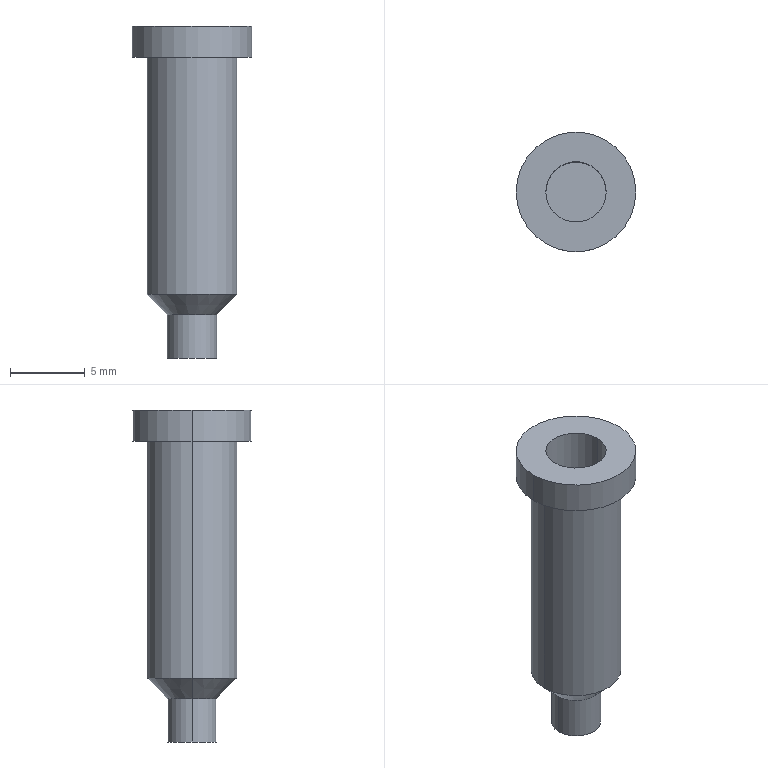Part | NX | features solid 2 | 1 solid | 14 faces | box 8 x 8 x 22.2 mm | volume 371.979 mm3 | cylinder 8 | plane 4 | cone 2 | commonest cylinder face diameters 3.3 x2 4.04 x2 6 x2 8 x2
STEP:
#1=CARTESIAN_POINT('',(-284.273,891.104,-19.1));
#2=VERTEX_POINT('',#1);
#3=CARTESIAN_POINT('',(-287.573,891.104,-19.1));
#4=VERTEX_POINT('',#3);
#5=CARTESIAN_POINT('',(-285.923,891.104,-19.1));
#6=DIRECTION('',(0.,0.,1.));
#7=DIRECTION('',(1.,0.,0.));
#8=AXIS2_PLACEMENT_3D('',#5,#6,#7);
#9=CIRCLE('',#8,1.65);
#10=EDGE_CURVE('',#2,#4,#9,.T.);
#11=ORIENTED_EDGE('',*,*,#10,.F.);
#12=CARTESIAN_POINT('',(-285.923,891.104,-19.1));
#13=DIRECTION('',(0.,0.,1.));
#14=DIRECTION('',(-1.,0.,0.));
#15=AXIS2_PLACEMENT_3D('',#12,#13,#14);
#16=CIRCLE('',#15,1.65);
#17=EDGE_CURVE('',#4,#2,#16,.T.);
#18=ORIENTED_EDGE('',*,*,#17,.F.);
#19=EDGE_LOOP('',(#11,#18));
#20=FACE_BOUND('',#19,.T.);
#21=CARTESIAN_POINT('',(-285.923,891.104,-19.1));
#22=DIRECTION('',(0.,0.,-1.));
#23=DIRECTION('',(-1.,0.,0.));
#24=AXIS2_PLACEMENT_3D('',#21,#22,#23);
#25=PLANE('',#24);
#26=ADVANCED_FACE('',(#20),#25,.T.);
#27=ORIENTED_EDGE('',*,*,#17,.T.);
#28=CARTESIAN_POINT('',(-284.273,891.104,-16.2));
#29=VERTEX_POINT('',#28);
#30=CARTESIAN_POINT('',(-284.273,891.104,-19.1));
#31=DIRECTION('',(0.,0.,1.));
#32=VECTOR('',#31,1000.);
#33=LINE('',#30,#32);
#34=EDGE_CURVE('',#29,#2,#33,.F.);
#35=ORIENTED_EDGE('',*,*,#34,.F.);
#36=CARTESIAN_POINT('',(-287.573,891.104,-16.2));
#37=VERTEX_POINT('',#36);
#38=CARTESIAN_POINT('',(-285.923,891.104,-16.2));
#39=DIRECTION('',(0.,0.,-1.));
#40=DIRECTION('',(1.,0.,0.));
#41=AXIS2_PLACEMENT_3D('',#38,#39,#40);
#42=CIRCLE('',#41,1.65);
#43=EDGE_CURVE('',#29,#37,#42,.T.);
#44=ORIENTED_EDGE('',*,*,#43,.T.);
#45=CARTESIAN_POINT('',(-287.573,891.104,-19.1));
#46=DIRECTION('',(0.,0.,1.));
#47=VECTOR('',#46,1000.);
#48=LINE('',#45,#47);
#49=EDGE_CURVE('',#4,#37,#48,.T.);
#50=ORIENTED_EDGE('',*,*,#49,.F.);
#51=EDGE_LOOP('',(#27,#35,#44,#50));
#52=FACE_BOUND('',#51,.T.);
#53=CARTESIAN_POINT('',(-285.923,891.104,4.21));
#54=DIRECTION('',(0.,0.,-1.));
#55=DIRECTION('',(-1.,0.,0.));
#56=AXIS2_PLACEMENT_3D('',#53,#54,#55);
#57=CYLINDRICAL_SURFACE('',#56,1.65);
#58=ADVANCED_FACE('',(#52),#57,.T.);
#59=CARTESIAN_POINT('',(-285.923,891.104,-16.2));
#60=DIRECTION('',(0.,0.,-1.));
#61=DIRECTION('',(-1.,0.,0.));
#62=AXIS2_PLACEMENT_3D('',#59,#60,#61);
#63=CIRCLE('',#62,1.65);
#64=EDGE_CURVE('',#37,#29,#63,.T.);
#65=ORIENTED_EDGE('',*,*,#64,.T.);
#66=ORIENTED_EDGE('',*,*,#34,.T.);
#67=ORIENTED_EDGE('',*,*,#10,.T.);
#68=ORIENTED_EDGE('',*,*,#49,.T.);
#69=EDGE_LOOP('',(#65,#66,#67,#68));
#70=FACE_BOUND('',#69,.T.);
#71=CARTESIAN_POINT('',(-285.923,891.104,4.21));
#72=DIRECTION('',(0.,0.,-1.));
#73=DIRECTION('',(-1.,0.,0.));
#74=AXIS2_PLACEMENT_3D('',#71,#72,#73);
#75=CYLINDRICAL_SURFACE('',#74,1.65);
#76=ADVANCED_FACE('',(#70),#75,.T.);
#77=CARTESIAN_POINT('',(-282.923,891.104,-14.85));
#78=VERTEX_POINT('',#77);
#79=CARTESIAN_POINT('',(-288.923,891.104,-14.85));
#80=VERTEX_POINT('',#79);
#81=CARTESIAN_POINT('',(-285.923,891.104,-14.85));
#82=DIRECTION('',(0.,0.,1.));
#83=DIRECTION('',(1.,0.,0.));
#84=AXIS2_PLACEMENT_3D('',#81,#82,#83);
#85=CIRCLE('',#84,3.);
#86=EDGE_CURVE('',#78,#80,#85,.T.);
#87=ORIENTED_EDGE('',*,*,#86,.F.);
#88=CARTESIAN_POINT('',(-284.273,891.104,-16.2));
#89=DIRECTION('',(0.7071,0.,0.7071));
#90=VECTOR('',#89,1000.);
#91=LINE('',#88,#90);
#92=EDGE_CURVE('',#29,#78,#91,.T.);
#93=ORIENTED_EDGE('',*,*,#92,.F.);
#94=ORIENTED_EDGE('',*,*,#64,.F.);
#95=CARTESIAN_POINT('',(-287.573,891.104,-16.2));
#96=DIRECTION('',(-0.7071,0.,0.7071));
#97=VECTOR('',#96,1000.);
#98=LINE('',#95,#97);
#99=EDGE_CURVE('',#80,#37,#98,.F.);
#100=ORIENTED_EDGE('',*,*,#99,.F.);
#101=EDGE_LOOP('',(#87,#93,#94,#100));
#102=FACE_BOUND('',#101,.T.);
#103=CARTESIAN_POINT('',(-285.923,891.104,-15.525));
#104=DIRECTION('',(0.,0.,1.));
#105=DIRECTION('',(1.,0.,0.));
#106=AXIS2_PLACEMENT_3D('',#103,#104,#105);
#107=CONICAL_SURFACE('',#106,2.325,0.7854);
#108=ADVANCED_FACE('',(#102),#107,.T.);
#109=ORIENTED_EDGE('',*,*,#43,.F.);
#110=ORIENTED_EDGE('',*,*,#92,.T.);
#111=CARTESIAN_POINT('',(-285.923,891.104,-14.85));
#112=DIRECTION('',(0.,0.,1.));
#113=DIRECTION('',(-1.,0.,0.));
#114=AXIS2_PLACEMENT_3D('',#111,#112,#113);
#115=CIRCLE('',#114,3.);
#116=EDGE_CURVE('',#80,#78,#115,.T.);
#117=ORIENTED_EDGE('',*,*,#116,.F.);
#118=ORIENTED_EDGE('',*,*,#99,.T.);
#119=EDGE_LOOP('',(#109,#110,#117,#118));
#120=FACE_BOUND('',#119,.T.);
#121=CARTESIAN_POINT('',(-285.923,891.104,-15.525));
#122=DIRECTION('',(0.,0.,1.));
#123=DIRECTION('',(1.,0.,0.));
#124=AXIS2_PLACEMENT_3D('',#121,#122,#123);
#125=CONICAL_SURFACE('',#124,2.325,0.7854);
#126=ADVANCED_FACE('',(#120),#125,.T.);
#127=ORIENTED_EDGE('',*,*,#116,.T.);
#128=CARTESIAN_POINT('',(-282.923,891.104,1.));
#129=VERTEX_POINT('',#128);
#130=CARTESIAN_POINT('',(-282.923,891.104,-14.85));
#131=DIRECTION('',(0.,0.,1.));
#132=VECTOR('',#131,1000.);
#133=LINE('',#130,#132);
#134=EDGE_CURVE('',#78,#129,#133,.T.);
#135=ORIENTED_EDGE('',*,*,#134,.T.);
#136=CARTESIAN_POINT('',(-288.923,891.104,1.));
#137=VERTEX_POINT('',#136);
#138=CARTESIAN_POINT('',(-285.923,891.104,1.));
#139=DIRECTION('',(0.,0.,-1.));
#140=DIRECTION('',(1.,0.,0.));
#141=AXIS2_PLACEMENT_3D('',#138,#139,#140);
#142=CIRCLE('',#141,3.);
#143=EDGE_CURVE('',#129,#137,#142,.T.);
#144=ORIENTED_EDGE('',*,*,#143,.T.);
#145=CARTESIAN_POINT('',(-288.923,891.104,-14.85));
#146=DIRECTION('',(0.,0.,1.));
#147=VECTOR('',#146,1000.);
#148=LINE('',#145,#147);
#149=EDGE_CURVE('',#137,#80,#148,.F.);
#150=ORIENTED_EDGE('',*,*,#149,.T.);
#151=EDGE_LOOP('',(#127,#135,#144,#150));
#152=FACE_BOUND('',#151,.T.);
#153=CARTESIAN_POINT('',(-285.923,891.104,4.21));
#154=DIRECTION('',(0.,0.,-1.));
#155=DIRECTION('',(-1.,0.,0.));
#156=AXIS2_PLACEMENT_3D('',#153,#154,#155);
#157=CYLINDRICAL_SURFACE('',#156,3.);
#158=ADVANCED_FACE('',(#152),#157,.T.);
#159=CARTESIAN_POINT('',(-285.923,891.104,1.));
#160=DIRECTION('',(0.,0.,-1.));
#161=DIRECTION('',(-1.,0.,0.));
#162=AXIS2_PLACEMENT_3D('',#159,#160,#161);
#163=CIRCLE('',#162,3.);
#164=EDGE_CURVE('',#137,#129,#163,.T.);
#165=ORIENTED_EDGE('',*,*,#164,.T.);
#166=ORIENTED_EDGE('',*,*,#134,.F.);
#167=ORIENTED_EDGE('',*,*,#86,.T.);
#168=ORIENTED_EDGE('',*,*,#149,.F.);
#169=EDGE_LOOP('',(#165,#166,#167,#168));
#170=FACE_BOUND('',#169,.T.);
#171=CARTESIAN_POINT('',(-285.923,891.104,4.21));
#172=DIRECTION('',(0.,0.,-1.));
#173=DIRECTION('',(-1.,0.,0.));
#174=AXIS2_PLACEMENT_3D('',#171,#172,#173);
#175=CYLINDRICAL_SURFACE('',#174,3.);
#176=ADVANCED_FACE('',(#170),#175,.T.);
#177=CARTESIAN_POINT('',(-281.923,891.104,1.));
#178=VERTEX_POINT('',#177);
#179=CARTESIAN_POINT('',(-289.923,891.104,1.));
#180=VERTEX_POINT('',#179);
#181=CARTESIAN_POINT('',(-285.923,891.104,1.));
#182=DIRECTION('',(0.,0.,1.));
#183=DIRECTION('',(1.,0.,0.));
#184=AXIS2_PLACEMENT_3D('',#181,#182,#183);
#185=CIRCLE('',#184,4.);
#186=EDGE_CURVE('',#178,#180,#185,.T.);
#187=ORIENTED_EDGE('',*,*,#186,.F.);
#188=CARTESIAN_POINT('',(-285.923,891.104,1.));
#189=DIRECTION('',(0.,0.,1.));
#190=DIRECTION('',(-1.,0.,0.));
#191=AXIS2_PLACEMENT_3D('',#188,#189,#190);
#192=CIRCLE('',#191,4.);
#193=EDGE_CURVE('',#180,#178,#192,.T.);
#194=ORIENTED_EDGE('',*,*,#193,.F.);
#195=EDGE_LOOP('',(#187,#194));
#196=FACE_BOUND('',#195,.T.);
#197=ORIENTED_EDGE('',*,*,#143,.F.);
#198=ORIENTED_EDGE('',*,*,#164,.F.);
#199=EDGE_LOOP('',(#197,#198));
#200=FACE_BOUND('',#199,.T.);
#201=CARTESIAN_POINT('',(-285.923,891.104,1.));
#202=DIRECTION('',(0.,0.,-1.));
#203=DIRECTION('',(-1.,0.,0.));
#204=AXIS2_PLACEMENT_3D('',#201,#202,#203);
#205=PLANE('',#204);
#206=ADVANCED_FACE('',(#196,#200),#205,.T.);
#207=ORIENTED_EDGE('',*,*,#193,.T.);
#208=CARTESIAN_POINT('',(-281.923,891.104,3.1));
#209=VERTEX_POINT('',#208);
#210=CARTESIAN_POINT('',(-281.923,891.104,1.));
#211=DIRECTION('',(0.,0.,1.));
#212=VECTOR('',#211,1000.);
#213=LINE('',#210,#212);
#214=EDGE_CURVE('',#178,#209,#213,.T.);
#215=ORIENTED_EDGE('',*,*,#214,.T.);
#216=CARTESIAN_POINT('',(-289.923,891.104,3.1));
#217=VERTEX_POINT('',#216);
#218=CARTESIAN_POINT('',(-285.923,891.104,3.1));
#219=DIRECTION('',(0.,0.,-1.));
#220=DIRECTION('',(1.,0.,0.));
#221=AXIS2_PLACEMENT_3D('',#218,#219,#220);
#222=CIRCLE('',#221,4.);
#223=EDGE_CURVE('',#209,#217,#222,.T.);
#224=ORIENTED_EDGE('',*,*,#223,.T.);
#225=CARTESIAN_POINT('',(-289.923,891.104,1.));
#226=DIRECTION('',(0.,0.,1.));
#227=VECTOR('',#226,1000.);
#228=LINE('',#225,#227);
#229=EDGE_CURVE('',#217,#180,#228,.F.);
#230=ORIENTED_EDGE('',*,*,#229,.T.);
#231=EDGE_LOOP('',(#207,#215,#224,#230));
#232=FACE_BOUND('',#231,.T.);
#233=CARTESIAN_POINT('',(-285.923,891.104,4.21));
#234=DIRECTION('',(0.,0.,-1.));
#235=DIRECTION('',(-1.,0.,0.));
#236=AXIS2_PLACEMENT_3D('',#233,#234,#235);
#237=CYLINDRICAL_SURFACE('',#236,4.);
#238=ADVANCED_FACE('',(#232),#237,.T.);
#239=CARTESIAN_POINT('',(-285.923,891.104,3.1));
#240=DIRECTION('',(0.,0.,-1.));
#241=DIRECTION('',(-1.,0.,0.));
#242=AXIS2_PLACEMENT_3D('',#239,#240,#241);
#243=CIRCLE('',#242,4.);
#244=EDGE_CURVE('',#217,#209,#243,.T.);
#245=ORIENTED_EDGE('',*,*,#244,.T.);
#246=ORIENTED_EDGE('',*,*,#214,.F.);
#247=ORIENTED_EDGE('',*,*,#186,.T.);
#248=ORIENTED_EDGE('',*,*,#229,.F.);
#249=EDGE_LOOP('',(#245,#246,#247,#248));
#250=FACE_BOUND('',#249,.T.);
#251=CARTESIAN_POINT('',(-285.923,891.104,4.21));
#252=DIRECTION('',(0.,0.,-1.));
#253=DIRECTION('',(-1.,0.,0.));
#254=AXIS2_PLACEMENT_3D('',#251,#252,#253);
#255=CYLINDRICAL_SURFACE('',#254,4.);
#256=ADVANCED_FACE('',(#250),#255,.T.);
#257=ORIENTED_EDGE('',*,*,#244,.F.);
#258=ORIENTED_EDGE('',*,*,#223,.F.);
#259=EDGE_LOOP('',(#257,#258));
#260=FACE_BOUND('',#259,.T.);
#261=CARTESIAN_POINT('',(-287.943,891.104,3.1));
#262=VERTEX_POINT('',#261);
#263=CARTESIAN_POINT('',(-283.903,891.104,3.1));
#264=VERTEX_POINT('',#263);
#265=CARTESIAN_POINT('',(-285.923,891.104,3.1));
#266=DIRECTION('',(0.,0.,1.));
#267=DIRECTION('',(-1.,0.,0.));
#268=AXIS2_PLACEMENT_3D('',#265,#266,#267);
#269=CIRCLE('',#268,2.02);
#270=EDGE_CURVE('',#262,#264,#269,.T.);
#271=ORIENTED_EDGE('',*,*,#270,.F.);
#272=CARTESIAN_POINT('',(-285.923,891.104,3.1));
#273=DIRECTION('',(0.,0.,1.));
#274=DIRECTION('',(1.,0.,0.));
#275=AXIS2_PLACEMENT_3D('',#272,#273,#274);
#276=CIRCLE('',#275,2.02);
#277=EDGE_CURVE('',#264,#262,#276,.T.);
#278=ORIENTED_EDGE('',*,*,#277,.F.);
#279=EDGE_LOOP('',(#271,#278));
#280=FACE_BOUND('',#279,.T.);
#281=CARTESIAN_POINT('',(-285.923,891.104,3.1));
#282=DIRECTION('',(0.,0.,-1.));
#283=DIRECTION('',(-1.,0.,0.));
#284=AXIS2_PLACEMENT_3D('',#281,#282,#283);
#285=PLANE('',#284);
#286=ADVANCED_FACE('',(#260,#280),#285,.F.);
#287=CARTESIAN_POINT('',(-287.943,891.104,-14.85));
#288=VERTEX_POINT('',#287);
#289=CARTESIAN_POINT('',(-287.943,891.104,3.1));
#290=DIRECTION('',(0.,0.,-1.));
#291=VECTOR('',#290,1000.);
#292=LINE('',#289,#291);
#293=EDGE_CURVE('',#262,#288,#292,.T.);
#294=ORIENTED_EDGE('',*,*,#293,.T.);
#295=CARTESIAN_POINT('',(-283.903,891.104,-14.85));
#296=VERTEX_POINT('',#295);
#297=CARTESIAN_POINT('',(-285.923,891.104,-14.85));
#298=DIRECTION('',(0.,0.,-1.));
#299=DIRECTION('',(-1.,0.,0.));
#300=AXIS2_PLACEMENT_3D('',#297,#298,#299);
#301=CIRCLE('',#300,2.02);
#302=EDGE_CURVE('',#288,#296,#301,.T.);
#303=ORIENTED_EDGE('',*,*,#302,.T.);
#304=CARTESIAN_POINT('',(-283.903,891.104,3.1));
#305=DIRECTION('',(0.,0.,-1.));
#306=VECTOR('',#305,1000.);
#307=LINE('',#304,#306);
#308=EDGE_CURVE('',#296,#264,#307,.F.);
#309=ORIENTED_EDGE('',*,*,#308,.T.);
#310=ORIENTED_EDGE('',*,*,#277,.T.);
#311=EDGE_LOOP('',(#294,#303,#309,#310));
#312=FACE_BOUND('',#311,.T.);
#313=CARTESIAN_POINT('',(-285.923,891.104,3.1));
#314=DIRECTION('',(0.,0.,1.));
#315=DIRECTION('',(-1.,0.,0.));
#316=AXIS2_PLACEMENT_3D('',#313,#314,#315);
#317=CYLINDRICAL_SURFACE('',#316,2.02);
#318=ADVANCED_FACE('',(#312),#317,.F.);
#319=ORIENTED_EDGE('',*,*,#308,.F.);
#320=CARTESIAN_POINT('',(-285.923,891.104,-14.85));
#321=DIRECTION('',(0.,0.,-1.));
#322=DIRECTION('',(1.,0.,0.));
#323=AXIS2_PLACEMENT_3D('',#320,#321,#322);
#324=CIRCLE('',#323,2.02);
#325=EDGE_CURVE('',#296,#288,#324,.T.);
#326=ORIENTED_EDGE('',*,*,#325,.T.);
#327=ORIENTED_EDGE('',*,*,#293,.F.);
#328=ORIENTED_EDGE('',*,*,#270,.T.);
#329=EDGE_LOOP('',(#319,#326,#327,#328));
#330=FACE_BOUND('',#329,.T.);
#331=CARTESIAN_POINT('',(-285.923,891.104,3.1));
#332=DIRECTION('',(0.,0.,1.));
#333=DIRECTION('',(-1.,0.,0.));
#334=AXIS2_PLACEMENT_3D('',#331,#332,#333);
#335=CYLINDRICAL_SURFACE('',#334,2.02);
#336=ADVANCED_FACE('',(#330),#335,.F.);
#337=ORIENTED_EDGE('',*,*,#325,.F.);
#338=ORIENTED_EDGE('',*,*,#302,.F.);
#339=EDGE_LOOP('',(#337,#338));
#340=FACE_BOUND('',#339,.T.);
#341=CARTESIAN_POINT('',(-285.923,891.104,-14.85));
#342=DIRECTION('',(0.,0.,1.));
#343=DIRECTION('',(-1.,0.,0.));
#344=AXIS2_PLACEMENT_3D('',#341,#342,#343);
#345=PLANE('',#344);
#346=ADVANCED_FACE('',(#340),#345,.T.);
#347=CLOSED_SHELL('',(#26,#58,#76,#108,#126,#158,#176,#206,#238,#256,#286,#318,#336,#346));
#348=MANIFOLD_SOLID_BREP('',#347);
#349=(LENGTH_UNIT()NAMED_UNIT(*)SI_UNIT(.MILLI.,.METRE.));
#350=UNCERTAINTY_MEASURE_WITH_UNIT(LENGTH_MEASURE(0.00001),#349,'','');
#351=(NAMED_UNIT(*)PLANE_ANGLE_UNIT()SI_UNIT($,.RADIAN.));
#352=(NAMED_UNIT(*)SI_UNIT($,.STERADIAN.)SOLID_ANGLE_UNIT());
#353=(GEOMETRIC_REPRESENTATION_CONTEXT(3)GLOBAL_UNCERTAINTY_ASSIGNED_CONTEXT((#350))GLOBAL_UNIT_ASSIGNED_CONTEXT((#349,#351,#352))REPRESENTATION_CONTEXT('',''));
#354=ADVANCED_BREP_SHAPE_REPRESENTATION('',(#348),#353);